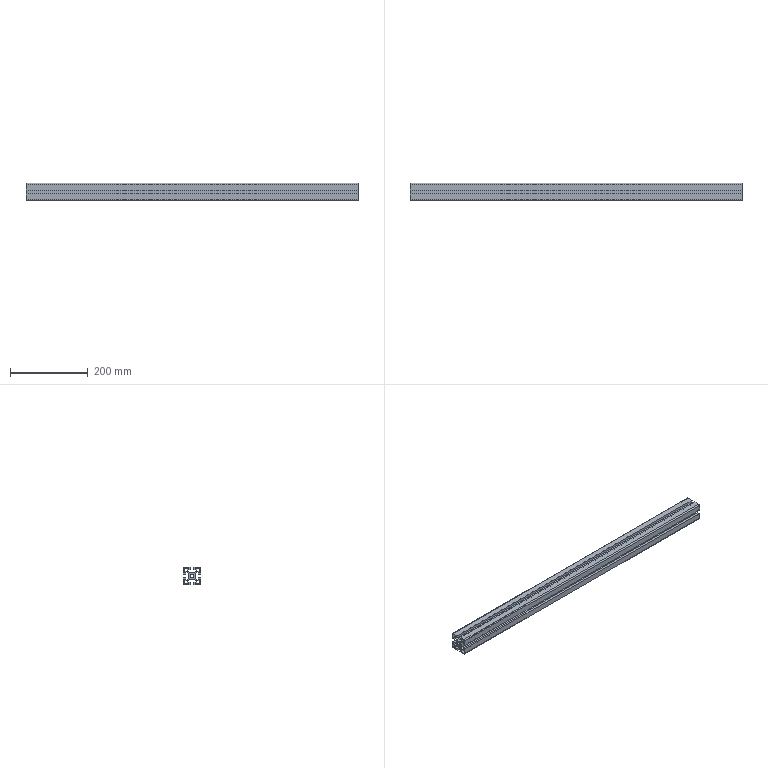Part | STEP file | 1_2 | 1 solid | 87 faces | box 855 x 45 x 45 mm | volume 699170 mm3 | plane 78 | cylinder 9 | commonest cylinder face diameters 2 x4 6 x4 10 x1